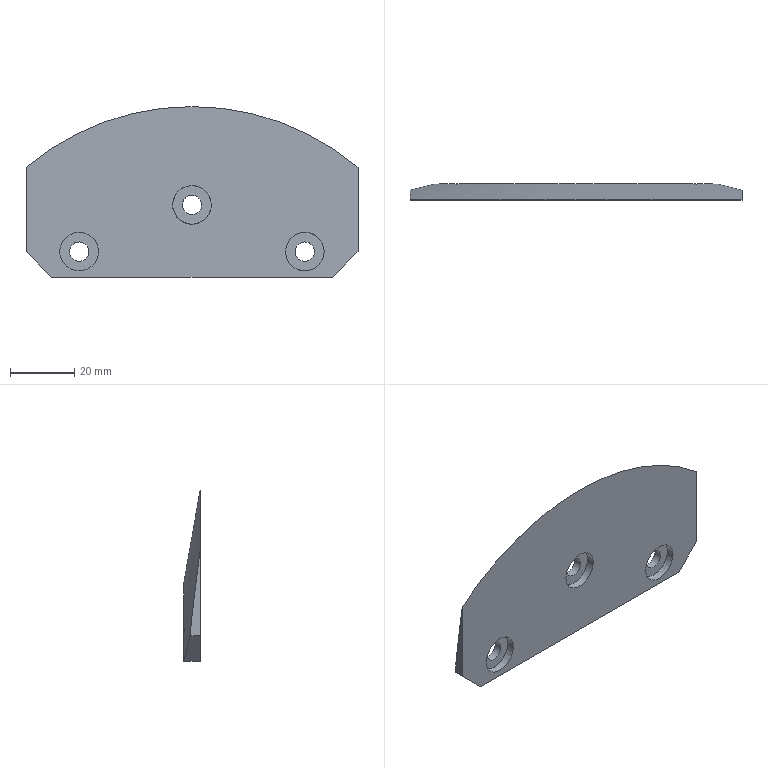Part | NX | features DATUM_CSYS 7, SKETCH 6, EXTRUDE 4, EXTRACT_DATUM_AXIS 3, EXTRACT_DATUM_PLANE 3, EXTRACT_FACE 3, EXTRACT_STRING 3, HOLE PACKAGE 3, SIMPLE HOLE 3, Instance Feature 2, CHAMFER 1, Pattern Feature 1, SWP104 1 | 1 solid | 17 faces | box 103 x 5 x 53 mm | volume 14704 mm3 | plane 10 | cylinder 6 | cone 1 | commonest cylinder face diameters 6 x3 12 x3
STEP:
#1=CARTESIAN_POINT('',(-35.,0.,41.));
#2=VERTEX_POINT('',#1);
#3=CARTESIAN_POINT('',(-35.,0.,35.));
#4=DIRECTION('',(0.,1.,0.));
#5=DIRECTION('',(0.,0.,1.));
#6=AXIS2_PLACEMENT_3D('',#3,#4,#5);
#7=CIRCLE('',#6,6.);
#8=EDGE_CURVE('',#2,#2,#7,.F.);
#9=ORIENTED_EDGE('',*,*,#8,.F.);
#10=EDGE_LOOP('',(#9));
#11=FACE_BOUND('',#10,.T.);
#12=CARTESIAN_POINT('',(0.,0.,55.497));
#13=VERTEX_POINT('',#12);
#14=CARTESIAN_POINT('',(0.,0.,49.497));
#15=DIRECTION('',(0.,1.,0.));
#16=DIRECTION('',(0.,0.,1.));
#17=AXIS2_PLACEMENT_3D('',#14,#15,#16);
#18=CIRCLE('',#17,6.);
#19=EDGE_CURVE('',#13,#13,#18,.F.);
#20=ORIENTED_EDGE('',*,*,#19,.F.);
#21=EDGE_LOOP('',(#20));
#22=FACE_BOUND('',#21,.T.);
#23=CARTESIAN_POINT('',(35.,0.,41.));
#24=VERTEX_POINT('',#23);
#25=CARTESIAN_POINT('',(35.,0.,35.));
#26=DIRECTION('',(0.,1.,0.));
#27=DIRECTION('',(0.,0.,1.));
#28=AXIS2_PLACEMENT_3D('',#25,#26,#27);
#29=CIRCLE('',#28,6.);
#30=EDGE_CURVE('',#24,#24,#29,.F.);
#31=ORIENTED_EDGE('',*,*,#30,.F.);
#32=EDGE_LOOP('',(#31));
#33=FACE_BOUND('',#32,.T.);
#34=CARTESIAN_POINT('',(43.5,0.,27.));
#35=VERTEX_POINT('',#34);
#36=CARTESIAN_POINT('',(-43.5,0.,27.));
#37=VERTEX_POINT('',#36);
#38=CARTESIAN_POINT('',(0.,0.,27.));
#39=DIRECTION('',(-1.,0.,0.));
#40=VECTOR('',#39,1000.);
#41=LINE('',#38,#40);
#42=EDGE_CURVE('',#35,#37,#41,.T.);
#43=ORIENTED_EDGE('',*,*,#42,.F.);
#44=CARTESIAN_POINT('',(51.5,0.,35.));
#45=VERTEX_POINT('',#44);
#46=CARTESIAN_POINT('',(43.5,0.,27.));
#47=DIRECTION('',(-0.7071,0.,-0.7071));
#48=VECTOR('',#47,1000.);
#49=LINE('',#46,#48);
#50=EDGE_CURVE('',#35,#45,#49,.F.);
#51=ORIENTED_EDGE('',*,*,#50,.T.);
#52=CARTESIAN_POINT('',(51.5,0.,61.219));
#53=VERTEX_POINT('',#52);
#54=CARTESIAN_POINT('',(51.5,0.,80.));
#55=DIRECTION('',(0.,0.,-1.));
#56=VECTOR('',#55,1000.);
#57=LINE('',#54,#56);
#58=EDGE_CURVE('',#53,#45,#57,.T.);
#59=ORIENTED_EDGE('',*,*,#58,.F.);
#60=CARTESIAN_POINT('',(-51.5,0.,61.219));
#61=VERTEX_POINT('',#60);
#62=CARTESIAN_POINT('',(0.,0.,0.));
#63=DIRECTION('',(0.,-1.,0.));
#64=DIRECTION('',(0.,0.,-1.));
#65=AXIS2_PLACEMENT_3D('',#62,#63,#64);
#66=CIRCLE('',#65,80.);
#67=EDGE_CURVE('',#53,#61,#66,.T.);
#68=ORIENTED_EDGE('',*,*,#67,.T.);
#69=CARTESIAN_POINT('',(-51.5,0.,35.));
#70=VERTEX_POINT('',#69);
#71=CARTESIAN_POINT('',(-51.5,0.,80.));
#72=DIRECTION('',(0.,0.,1.));
#73=VECTOR('',#72,1000.);
#74=LINE('',#71,#73);
#75=EDGE_CURVE('',#70,#61,#74,.T.);
#76=ORIENTED_EDGE('',*,*,#75,.F.);
#77=CARTESIAN_POINT('',(-51.5,0.,35.));
#78=DIRECTION('',(-0.7071,0.,0.7071));
#79=VECTOR('',#78,1000.);
#80=LINE('',#77,#79);
#81=EDGE_CURVE('',#70,#37,#80,.F.);
#82=ORIENTED_EDGE('',*,*,#81,.T.);
#83=EDGE_LOOP('',(#43,#51,#59,#68,#76,#82));
#84=FACE_BOUND('',#83,.T.);
#85=CARTESIAN_POINT('',(0.,0.,80.));
#86=DIRECTION('',(0.,1.,0.));
#87=DIRECTION('',(0.,0.,1.));
#88=AXIS2_PLACEMENT_3D('',#85,#86,#87);
#89=PLANE('',#88);
#90=ADVANCED_FACE('',(#11,#22,#33,#84),#89,.F.);
#91=CARTESIAN_POINT('',(-38.,5.,34.972));
#92=VERTEX_POINT('',#91);
#93=CARTESIAN_POINT('',(-43.823,5.,27.323));
#94=VERTEX_POINT('',#93);
#95=CARTESIAN_POINT('',(0.,5.,0.));
#96=DIRECTION('',(0.,-1.,0.));
#97=DIRECTION('',(0.,0.,-1.));
#98=AXIS2_PLACEMENT_3D('',#95,#96,#97);
#99=CIRCLE('',#98,51.644);
#100=EDGE_CURVE('',#92,#94,#99,.T.);
#101=ORIENTED_EDGE('',*,*,#100,.F.);
#102=CARTESIAN_POINT('',(-34.972,5.,38.));
#103=VERTEX_POINT('',#102);
#104=CARTESIAN_POINT('',(-35.,5.,35.));
#105=DIRECTION('',(0.,-1.,0.));
#106=DIRECTION('',(0.,0.,-1.));
#107=AXIS2_PLACEMENT_3D('',#104,#105,#106);
#108=CIRCLE('',#107,3.);
#109=EDGE_CURVE('',#92,#103,#108,.T.);
#110=ORIENTED_EDGE('',*,*,#109,.T.);
#111=CARTESIAN_POINT('',(-2.141,5.,51.599));
#112=VERTEX_POINT('',#111);
#113=CARTESIAN_POINT('',(0.,5.,0.));
#114=DIRECTION('',(0.,-1.,0.));
#115=DIRECTION('',(0.,0.,-1.));
#116=AXIS2_PLACEMENT_3D('',#113,#114,#115);
#117=CIRCLE('',#116,51.644);
#118=EDGE_CURVE('',#112,#103,#117,.T.);
#119=ORIENTED_EDGE('',*,*,#118,.F.);
#120=CARTESIAN_POINT('',(2.141,5.,51.599));
#121=VERTEX_POINT('',#120);
#122=CARTESIAN_POINT('',(0.,5.,49.497));
#123=DIRECTION('',(0.,-1.,0.));
#124=DIRECTION('',(0.,0.,-1.));
#125=AXIS2_PLACEMENT_3D('',#122,#123,#124);
#126=CIRCLE('',#125,3.);
#127=EDGE_CURVE('',#112,#121,#126,.T.);
#128=ORIENTED_EDGE('',*,*,#127,.T.);
#129=CARTESIAN_POINT('',(34.972,5.,38.));
#130=VERTEX_POINT('',#129);
#131=CARTESIAN_POINT('',(0.,5.,0.));
#132=DIRECTION('',(0.,-1.,0.));
#133=DIRECTION('',(0.,0.,-1.));
#134=AXIS2_PLACEMENT_3D('',#131,#132,#133);
#135=CIRCLE('',#134,51.644);
#136=EDGE_CURVE('',#130,#121,#135,.T.);
#137=ORIENTED_EDGE('',*,*,#136,.F.);
#138=CARTESIAN_POINT('',(38.,5.,34.972));
#139=VERTEX_POINT('',#138);
#140=CARTESIAN_POINT('',(35.,5.,35.));
#141=DIRECTION('',(0.,-1.,0.));
#142=DIRECTION('',(0.,0.,-1.));
#143=AXIS2_PLACEMENT_3D('',#140,#141,#142);
#144=CIRCLE('',#143,3.);
#145=EDGE_CURVE('',#130,#139,#144,.T.);
#146=ORIENTED_EDGE('',*,*,#145,.T.);
#147=CARTESIAN_POINT('',(43.823,5.,27.323));
#148=VERTEX_POINT('',#147);
#149=CARTESIAN_POINT('',(0.,5.,0.));
#150=DIRECTION('',(0.,-1.,0.));
#151=DIRECTION('',(0.,0.,-1.));
#152=AXIS2_PLACEMENT_3D('',#149,#150,#151);
#153=CIRCLE('',#152,51.644);
#154=EDGE_CURVE('',#148,#139,#153,.T.);
#155=ORIENTED_EDGE('',*,*,#154,.F.);
#156=CARTESIAN_POINT('',(43.5,5.,27.));
#157=VERTEX_POINT('',#156);
#158=CARTESIAN_POINT('',(43.5,5.,27.));
#159=DIRECTION('',(0.7071,0.,0.7071));
#160=VECTOR('',#159,1000.);
#161=LINE('',#158,#160);
#162=EDGE_CURVE('',#148,#157,#161,.F.);
#163=ORIENTED_EDGE('',*,*,#162,.T.);
#164=CARTESIAN_POINT('',(-43.5,5.,27.));
#165=VERTEX_POINT('',#164);
#166=CARTESIAN_POINT('',(0.,5.,27.));
#167=DIRECTION('',(1.,0.,0.));
#168=VECTOR('',#167,1000.);
#169=LINE('',#166,#168);
#170=EDGE_CURVE('',#165,#157,#169,.T.);
#171=ORIENTED_EDGE('',*,*,#170,.F.);
#172=CARTESIAN_POINT('',(-51.5,5.,35.));
#173=DIRECTION('',(0.7071,0.,-0.7071));
#174=VECTOR('',#173,1000.);
#175=LINE('',#172,#174);
#176=EDGE_CURVE('',#165,#94,#175,.F.);
#177=ORIENTED_EDGE('',*,*,#176,.T.);
#178=EDGE_LOOP('',(#101,#110,#119,#128,#137,#146,#155,#163,#171,#177));
#179=FACE_BOUND('',#178,.T.);
#180=CARTESIAN_POINT('',(0.,5.,0.));
#181=DIRECTION('',(0.,-1.,0.));
#182=DIRECTION('',(0.,0.,-1.));
#183=AXIS2_PLACEMENT_3D('',#180,#181,#182);
#184=PLANE('',#183);
#185=ADVANCED_FACE('',(#179),#184,.F.);
#186=ORIENTED_EDGE('',*,*,#118,.T.);
#187=CARTESIAN_POINT('',(-34.972,5.,38.));
#188=CARTESIAN_POINT('',(-35.77,4.904,38.007));
#189=CARTESIAN_POINT('',(-37.352,4.795,37.355));
#190=CARTESIAN_POINT('',(-38.007,4.904,35.77));
#191=CARTESIAN_POINT('',(-38.,5.,34.972));
#192=B_SPLINE_CURVE_WITH_KNOTS('',3,(#187,#188,#189,#190,#191),.UNSPECIFIED.,.F.,.F.,(4,1,4),(0.000001647,0.002379,0.004756),.UNSPECIFIED.);
#193=EDGE_CURVE('',#103,#92,#192,.T.);
#194=ORIENTED_EDGE('',*,*,#193,.T.);
#195=ORIENTED_EDGE('',*,*,#100,.T.);
#196=CARTESIAN_POINT('',(-51.5,3.127,35.));
#197=VERTEX_POINT('',#196);
#198=CARTESIAN_POINT('',(-43.823,5.,27.323));
#199=CARTESIAN_POINT('',(-46.383,4.378,29.883));
#200=CARTESIAN_POINT('',(-48.941,3.753,32.441));
#201=CARTESIAN_POINT('',(-51.5,3.127,35.));
#202=B_SPLINE_CURVE_WITH_KNOTS('',3,(#198,#199,#200,#201),.UNSPECIFIED.,.F.,.F.,(4,4),(0.,0.01102),.UNSPECIFIED.);
#203=EDGE_CURVE('',#94,#197,#202,.T.);
#204=ORIENTED_EDGE('',*,*,#203,.T.);
#205=CARTESIAN_POINT('',(-51.5,0.,61.219));
#206=CARTESIAN_POINT('',(-51.5,1.177,52.494));
#207=CARTESIAN_POINT('',(-51.5,2.259,43.758));
#208=CARTESIAN_POINT('',(-51.5,3.127,35.));
#209=B_SPLINE_CURVE_WITH_KNOTS('',3,(#205,#206,#207,#208),.UNSPECIFIED.,.F.,.F.,(4,4),(0.05125,0.07765),.UNSPECIFIED.);
#210=EDGE_CURVE('',#61,#197,#209,.T.);
#211=ORIENTED_EDGE('',*,*,#210,.F.);
#212=ORIENTED_EDGE('',*,*,#67,.F.);
#213=CARTESIAN_POINT('',(51.5,3.127,35.));
#214=VERTEX_POINT('',#213);
#215=CARTESIAN_POINT('',(51.5,3.127,35.));
#216=CARTESIAN_POINT('',(51.5,2.259,43.754));
#217=CARTESIAN_POINT('',(51.5,1.177,52.496));
#218=CARTESIAN_POINT('',(51.5,0.,61.219));
#219=B_SPLINE_CURVE_WITH_KNOTS('',3,(#215,#216,#217,#218),.UNSPECIFIED.,.F.,.F.,(4,4),(0.03998,0.06635),.UNSPECIFIED.);
#220=EDGE_CURVE('',#214,#53,#219,.T.);
#221=ORIENTED_EDGE('',*,*,#220,.F.);
#222=CARTESIAN_POINT('',(51.5,3.127,35.));
#223=CARTESIAN_POINT('',(48.941,3.753,32.441));
#224=CARTESIAN_POINT('',(46.383,4.378,29.883));
#225=CARTESIAN_POINT('',(43.823,5.,27.323));
#226=B_SPLINE_CURVE_WITH_KNOTS('',3,(#222,#223,#224,#225),.UNSPECIFIED.,.F.,.F.,(4,4),(0.,0.01102),.UNSPECIFIED.);
#227=EDGE_CURVE('',#214,#148,#226,.T.);
#228=ORIENTED_EDGE('',*,*,#227,.T.);
#229=ORIENTED_EDGE('',*,*,#154,.T.);
#230=CARTESIAN_POINT('',(38.,5.,34.972));
#231=CARTESIAN_POINT('',(38.007,4.904,35.77));
#232=CARTESIAN_POINT('',(37.355,4.795,37.352));
#233=CARTESIAN_POINT('',(35.77,4.904,38.007));
#234=CARTESIAN_POINT('',(34.972,5.,38.));
#235=B_SPLINE_CURVE_WITH_KNOTS('',3,(#230,#231,#232,#233,#234),.UNSPECIFIED.,.F.,.F.,(4,1,4),(0.000001647,0.002379,0.004756),.UNSPECIFIED.);
#236=EDGE_CURVE('',#139,#130,#235,.T.);
#237=ORIENTED_EDGE('',*,*,#236,.T.);
#238=ORIENTED_EDGE('',*,*,#136,.T.);
#239=CARTESIAN_POINT('',(2.141,5.,51.599));
#240=CARTESIAN_POINT('',(1.582,4.904,52.169));
#241=CARTESIAN_POINT('',(0.002182,4.795,52.826));
#242=CARTESIAN_POINT('',(-1.582,4.904,52.169));
#243=CARTESIAN_POINT('',(-2.141,5.,51.599));
#244=B_SPLINE_CURVE_WITH_KNOTS('',3,(#239,#240,#241,#242,#243),.UNSPECIFIED.,.F.,.F.,(4,1,4),(0.000001647,0.002379,0.004756),.UNSPECIFIED.);
#245=EDGE_CURVE('',#121,#112,#244,.T.);
#246=ORIENTED_EDGE('',*,*,#245,.T.);
#247=EDGE_LOOP('',(#186,#194,#195,#204,#211,#212,#221,#228,#229,#237,#238,#246));
#248=FACE_BOUND('',#247,.T.);
#249=CARTESIAN_POINT('',(0.,5.,0.));
#250=DIRECTION('',(0.,-1.,0.));
#251=DIRECTION('',(0.,0.,-1.));
#252=AXIS2_PLACEMENT_3D('',#249,#250,#251);
#253=CONICAL_SURFACE('',#252,51.644,1.396);
#254=ADVANCED_FACE('',(#248),#253,.T.);
#255=ORIENTED_EDGE('',*,*,#58,.T.);
#256=CARTESIAN_POINT('',(51.5,-104.,35.));
#257=DIRECTION('',(0.,1.,0.));
#258=VECTOR('',#257,1000.);
#259=LINE('',#256,#258);
#260=EDGE_CURVE('',#45,#214,#259,.T.);
#261=ORIENTED_EDGE('',*,*,#260,.T.);
#262=ORIENTED_EDGE('',*,*,#220,.T.);
#263=EDGE_LOOP('',(#255,#261,#262));
#264=FACE_BOUND('',#263,.T.);
#265=CARTESIAN_POINT('',(51.5,-104.,85.191));
#266=DIRECTION('',(1.,0.,0.));
#267=DIRECTION('',(0.,0.,-1.));
#268=AXIS2_PLACEMENT_3D('',#265,#266,#267);
#269=PLANE('',#268);
#270=ADVANCED_FACE('',(#264),#269,.T.);
#271=ORIENTED_EDGE('',*,*,#170,.T.);
#272=CARTESIAN_POINT('',(43.5,-104.,27.));
#273=DIRECTION('',(0.,-1.,0.));
#274=VECTOR('',#273,1000.);
#275=LINE('',#272,#274);
#276=EDGE_CURVE('',#157,#35,#275,.T.);
#277=ORIENTED_EDGE('',*,*,#276,.T.);
#278=ORIENTED_EDGE('',*,*,#42,.T.);
#279=CARTESIAN_POINT('',(-43.5,-104.,27.));
#280=DIRECTION('',(0.,1.,0.));
#281=VECTOR('',#280,1000.);
#282=LINE('',#279,#281);
#283=EDGE_CURVE('',#37,#165,#282,.T.);
#284=ORIENTED_EDGE('',*,*,#283,.T.);
#285=EDGE_LOOP('',(#271,#277,#278,#284));
#286=FACE_BOUND('',#285,.T.);
#287=CARTESIAN_POINT('',(51.5,-104.,27.));
#288=DIRECTION('',(0.,0.,-1.));
#289=DIRECTION('',(-1.,0.,0.));
#290=AXIS2_PLACEMENT_3D('',#287,#288,#289);
#291=PLANE('',#290);
#292=ADVANCED_FACE('',(#286),#291,.T.);
#293=ORIENTED_EDGE('',*,*,#210,.T.);
#294=CARTESIAN_POINT('',(-51.5,-104.,35.));
#295=DIRECTION('',(0.,-1.,0.));
#296=VECTOR('',#295,1000.);
#297=LINE('',#294,#296);
#298=EDGE_CURVE('',#197,#70,#297,.T.);
#299=ORIENTED_EDGE('',*,*,#298,.T.);
#300=ORIENTED_EDGE('',*,*,#75,.T.);
#301=EDGE_LOOP('',(#293,#299,#300));
#302=FACE_BOUND('',#301,.T.);
#303=CARTESIAN_POINT('',(-51.5,-104.,27.));
#304=DIRECTION('',(-1.,0.,0.));
#305=DIRECTION('',(0.,0.,1.));
#306=AXIS2_PLACEMENT_3D('',#303,#304,#305);
#307=PLANE('',#306);
#308=ADVANCED_FACE('',(#302),#307,.T.);
#309=ORIENTED_EDGE('',*,*,#227,.F.);
#310=ORIENTED_EDGE('',*,*,#260,.F.);
#311=ORIENTED_EDGE('',*,*,#50,.F.);
#312=ORIENTED_EDGE('',*,*,#276,.F.);
#313=ORIENTED_EDGE('',*,*,#162,.F.);
#314=EDGE_LOOP('',(#309,#310,#311,#312,#313));
#315=FACE_BOUND('',#314,.T.);
#316=CARTESIAN_POINT('',(43.5,-104.,27.));
#317=DIRECTION('',(-0.7071,0.,0.7071));
#318=DIRECTION('',(0.,-1.,0.));
#319=AXIS2_PLACEMENT_3D('',#316,#317,#318);
#320=PLANE('',#319);
#321=ADVANCED_FACE('',(#315),#320,.F.);
#322=ORIENTED_EDGE('',*,*,#176,.F.);
#323=ORIENTED_EDGE('',*,*,#283,.F.);
#324=ORIENTED_EDGE('',*,*,#81,.F.);
#325=ORIENTED_EDGE('',*,*,#298,.F.);
#326=ORIENTED_EDGE('',*,*,#203,.F.);
#327=EDGE_LOOP('',(#322,#323,#324,#325,#326));
#328=FACE_BOUND('',#327,.T.);
#329=CARTESIAN_POINT('',(-51.5,-104.,35.));
#330=DIRECTION('',(0.7071,0.,0.7071));
#331=DIRECTION('',(0.,-1.,0.));
#332=AXIS2_PLACEMENT_3D('',#329,#330,#331);
#333=PLANE('',#332);
#334=ADVANCED_FACE('',(#328),#333,.F.);
#335=CARTESIAN_POINT('',(35.,2.5,38.));
#336=VERTEX_POINT('',#335);
#337=CARTESIAN_POINT('',(35.,2.5,35.));
#338=DIRECTION('',(0.,1.,0.));
#339=DIRECTION('',(0.,0.,1.));
#340=AXIS2_PLACEMENT_3D('',#337,#338,#339);
#341=CIRCLE('',#340,3.);
#342=EDGE_CURVE('',#336,#336,#341,.T.);
#343=ORIENTED_EDGE('',*,*,#342,.F.);
#344=EDGE_LOOP('',(#343));
#345=FACE_BOUND('',#344,.T.);
#346=ORIENTED_EDGE('',*,*,#145,.F.);
#347=ORIENTED_EDGE('',*,*,#236,.F.);
#348=EDGE_LOOP('',(#346,#347));
#349=FACE_BOUND('',#348,.T.);
#350=CARTESIAN_POINT('',(35.,5.,35.));
#351=DIRECTION('',(0.,-1.,0.));
#352=DIRECTION('',(0.,0.,-1.));
#353=AXIS2_PLACEMENT_3D('',#350,#351,#352);
#354=CYLINDRICAL_SURFACE('',#353,3.);
#355=ADVANCED_FACE('',(#345,#349),#354,.F.);
#356=CARTESIAN_POINT('',(41.,2.5,35.));
#357=VERTEX_POINT('',#356);
#358=CARTESIAN_POINT('',(35.,2.5,35.));
#359=DIRECTION('',(0.,1.,0.));
#360=DIRECTION('',(1.,0.,0.));
#361=AXIS2_PLACEMENT_3D('',#358,#359,#360);
#362=CIRCLE('',#361,6.);
#363=EDGE_CURVE('',#357,#357,#362,.T.);
#364=ORIENTED_EDGE('',*,*,#363,.T.);
#365=EDGE_LOOP('',(#364));
#366=FACE_BOUND('',#365,.T.);
#367=ORIENTED_EDGE('',*,*,#30,.T.);
#368=EDGE_LOOP('',(#367));
#369=FACE_BOUND('',#368,.T.);
#370=CARTESIAN_POINT('',(35.,2.5,35.));
#371=DIRECTION('',(0.,-1.,0.));
#372=DIRECTION('',(0.,0.,-1.));
#373=AXIS2_PLACEMENT_3D('',#370,#371,#372);
#374=CYLINDRICAL_SURFACE('',#373,6.);
#375=ADVANCED_FACE('',(#366,#369),#374,.F.);
#376=ORIENTED_EDGE('',*,*,#363,.F.);
#377=EDGE_LOOP('',(#376));
#378=FACE_BOUND('',#377,.T.);
#379=ORIENTED_EDGE('',*,*,#342,.T.);
#380=EDGE_LOOP('',(#379));
#381=FACE_BOUND('',#380,.T.);
#382=CARTESIAN_POINT('',(35.,2.5,35.));
#383=DIRECTION('',(0.,1.,0.));
#384=DIRECTION('',(0.,0.,1.));
#385=AXIS2_PLACEMENT_3D('',#382,#383,#384);
#386=PLANE('',#385);
#387=ADVANCED_FACE('',(#378,#381),#386,.F.);
#388=CARTESIAN_POINT('',(0.,2.5,52.497));
#389=VERTEX_POINT('',#388);
#390=CARTESIAN_POINT('',(0.,2.5,49.497));
#391=DIRECTION('',(0.,1.,0.));
#392=DIRECTION('',(0.,0.,1.));
#393=AXIS2_PLACEMENT_3D('',#390,#391,#392);
#394=CIRCLE('',#393,3.);
#395=EDGE_CURVE('',#389,#389,#394,.T.);
#396=ORIENTED_EDGE('',*,*,#395,.F.);
#397=EDGE_LOOP('',(#396));
#398=FACE_BOUND('',#397,.T.);
#399=ORIENTED_EDGE('',*,*,#127,.F.);
#400=ORIENTED_EDGE('',*,*,#245,.F.);
#401=EDGE_LOOP('',(#399,#400));
#402=FACE_BOUND('',#401,.T.);
#403=CARTESIAN_POINT('',(0.,5.,49.497));
#404=DIRECTION('',(0.,-1.,0.));
#405=DIRECTION('',(0.,0.,-1.));
#406=AXIS2_PLACEMENT_3D('',#403,#404,#405);
#407=CYLINDRICAL_SURFACE('',#406,3.);
#408=ADVANCED_FACE('',(#398,#402),#407,.F.);
#409=CARTESIAN_POINT('',(4.243,2.5,53.74));
#410=VERTEX_POINT('',#409);
#411=CARTESIAN_POINT('',(0.,2.5,49.497));
#412=DIRECTION('',(0.,1.,0.));
#413=DIRECTION('',(0.7071,0.,0.7071));
#414=AXIS2_PLACEMENT_3D('',#411,#412,#413);
#415=CIRCLE('',#414,6.);
#416=EDGE_CURVE('',#410,#410,#415,.T.);
#417=ORIENTED_EDGE('',*,*,#416,.T.);
#418=EDGE_LOOP('',(#417));
#419=FACE_BOUND('',#418,.T.);
#420=ORIENTED_EDGE('',*,*,#19,.T.);
#421=EDGE_LOOP('',(#420));
#422=FACE_BOUND('',#421,.T.);
#423=CARTESIAN_POINT('',(0.,2.5,49.497));
#424=DIRECTION('',(0.,-1.,0.));
#425=DIRECTION('',(0.,0.,-1.));
#426=AXIS2_PLACEMENT_3D('',#423,#424,#425);
#427=CYLINDRICAL_SURFACE('',#426,6.);
#428=ADVANCED_FACE('',(#419,#422),#427,.F.);
#429=ORIENTED_EDGE('',*,*,#416,.F.);
#430=EDGE_LOOP('',(#429));
#431=FACE_BOUND('',#430,.T.);
#432=ORIENTED_EDGE('',*,*,#395,.T.);
#433=EDGE_LOOP('',(#432));
#434=FACE_BOUND('',#433,.T.);
#435=CARTESIAN_POINT('',(0.,2.5,49.497));
#436=DIRECTION('',(0.,1.,0.));
#437=DIRECTION('',(0.,0.,1.));
#438=AXIS2_PLACEMENT_3D('',#435,#436,#437);
#439=PLANE('',#438);
#440=ADVANCED_FACE('',(#431,#434),#439,.F.);
#441=CARTESIAN_POINT('',(-35.,2.5,38.));
#442=VERTEX_POINT('',#441);
#443=CARTESIAN_POINT('',(-35.,2.5,35.));
#444=DIRECTION('',(0.,1.,0.));
#445=DIRECTION('',(0.,0.,1.));
#446=AXIS2_PLACEMENT_3D('',#443,#444,#445);
#447=CIRCLE('',#446,3.);
#448=EDGE_CURVE('',#442,#442,#447,.T.);
#449=ORIENTED_EDGE('',*,*,#448,.F.);
#450=EDGE_LOOP('',(#449));
#451=FACE_BOUND('',#450,.T.);
#452=ORIENTED_EDGE('',*,*,#109,.F.);
#453=ORIENTED_EDGE('',*,*,#193,.F.);
#454=EDGE_LOOP('',(#452,#453));
#455=FACE_BOUND('',#454,.T.);
#456=CARTESIAN_POINT('',(-35.,5.,35.));
#457=DIRECTION('',(0.,-1.,0.));
#458=DIRECTION('',(0.,0.,-1.));
#459=AXIS2_PLACEMENT_3D('',#456,#457,#458);
#460=CYLINDRICAL_SURFACE('',#459,3.);
#461=ADVANCED_FACE('',(#451,#455),#460,.F.);
#462=CARTESIAN_POINT('',(-35.,2.5,41.));
#463=VERTEX_POINT('',#462);
#464=CARTESIAN_POINT('',(-35.,2.5,35.));
#465=DIRECTION('',(0.,1.,0.));
#466=DIRECTION('',(0.,0.,1.));
#467=AXIS2_PLACEMENT_3D('',#464,#465,#466);
#468=CIRCLE('',#467,6.);
#469=EDGE_CURVE('',#463,#463,#468,.T.);
#470=ORIENTED_EDGE('',*,*,#469,.T.);
#471=EDGE_LOOP('',(#470));
#472=FACE_BOUND('',#471,.T.);
#473=ORIENTED_EDGE('',*,*,#8,.T.);
#474=EDGE_LOOP('',(#473));
#475=FACE_BOUND('',#474,.T.);
#476=CARTESIAN_POINT('',(-35.,2.5,35.));
#477=DIRECTION('',(0.,-1.,0.));
#478=DIRECTION('',(0.,0.,-1.));
#479=AXIS2_PLACEMENT_3D('',#476,#477,#478);
#480=CYLINDRICAL_SURFACE('',#479,6.);
#481=ADVANCED_FACE('',(#472,#475),#480,.F.);
#482=ORIENTED_EDGE('',*,*,#469,.F.);
#483=EDGE_LOOP('',(#482));
#484=FACE_BOUND('',#483,.T.);
#485=ORIENTED_EDGE('',*,*,#448,.T.);
#486=EDGE_LOOP('',(#485));
#487=FACE_BOUND('',#486,.T.);
#488=CARTESIAN_POINT('',(-35.,2.5,35.));
#489=DIRECTION('',(0.,1.,0.));
#490=DIRECTION('',(0.,0.,1.));
#491=AXIS2_PLACEMENT_3D('',#488,#489,#490);
#492=PLANE('',#491);
#493=ADVANCED_FACE('',(#484,#487),#492,.F.);
#494=CLOSED_SHELL('',(#90,#185,#254,#270,#292,#308,#321,#334,#355,#375,#387,#408,#428,#440,#461,#481,#493));
#495=MANIFOLD_SOLID_BREP('',#494);
#496=(LENGTH_UNIT()NAMED_UNIT(*)SI_UNIT(.MILLI.,.METRE.));
#497=UNCERTAINTY_MEASURE_WITH_UNIT(LENGTH_MEASURE(0.0508),#496,'','');
#498=(NAMED_UNIT(*)PLANE_ANGLE_UNIT()SI_UNIT($,.RADIAN.));
#499=(NAMED_UNIT(*)SI_UNIT($,.STERADIAN.)SOLID_ANGLE_UNIT());
#500=(GEOMETRIC_REPRESENTATION_CONTEXT(3)GLOBAL_UNCERTAINTY_ASSIGNED_CONTEXT((#497))GLOBAL_UNIT_ASSIGNED_CONTEXT((#496,#498,#499))REPRESENTATION_CONTEXT('',''));
#501=ADVANCED_BREP_SHAPE_REPRESENTATION('',(#495),#500);